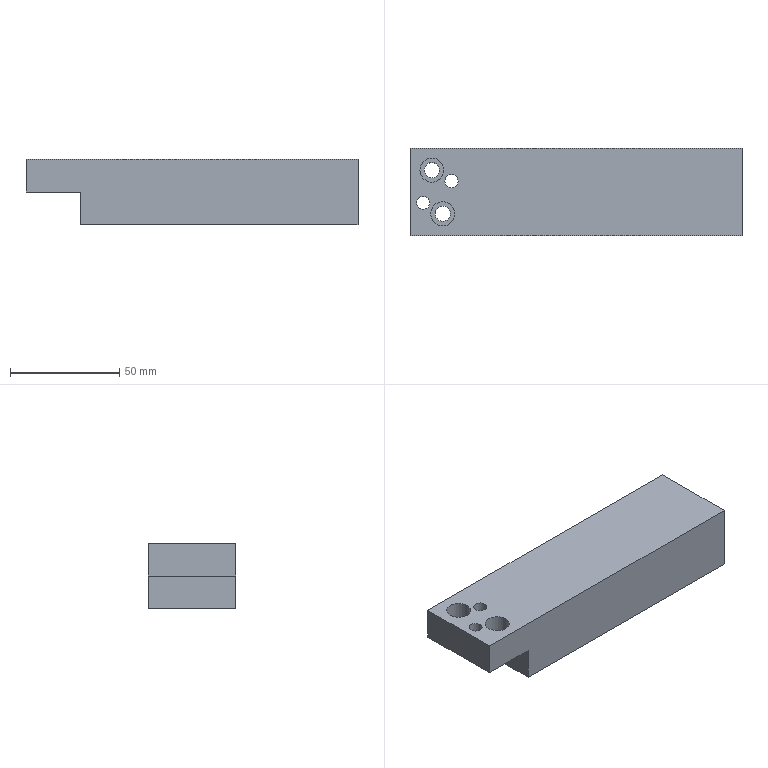Part | NX | features 22 2 | 1 solid | 16 faces | box 152 x 40 x 30 mm | volume 164266 mm3 | plane 10 | cylinder 6 | commonest cylinder face diameters 6.001 x2 7 x2 11 x2
STEP:
#1=CARTESIAN_POINT('',(905.,295.,-33.5));
#2=VERTEX_POINT('',#1);
#3=CARTESIAN_POINT('',(905.,255.,-33.5));
#4=VERTEX_POINT('',#3);
#5=CARTESIAN_POINT('',(905.,275.,-33.5));
#6=DIRECTION('',(0.,-1.,0.));
#7=VECTOR('',#6,1000.);
#8=LINE('',#5,#7);
#9=EDGE_CURVE('',#2,#4,#8,.T.);
#10=ORIENTED_EDGE('',*,*,#9,.F.);
#11=CARTESIAN_POINT('',(1032.,295.,-33.5));
#12=VERTEX_POINT('',#11);
#13=CARTESIAN_POINT('',(908.,295.,-33.5));
#14=DIRECTION('',(1.,0.,0.));
#15=VECTOR('',#14,1000.);
#16=LINE('',#13,#15);
#17=EDGE_CURVE('',#2,#12,#16,.T.);
#18=ORIENTED_EDGE('',*,*,#17,.T.);
#19=CARTESIAN_POINT('',(1032.,255.,-33.5));
#20=VERTEX_POINT('',#19);
#21=CARTESIAN_POINT('',(1032.,275.,-33.5));
#22=DIRECTION('',(0.,-1.,0.));
#23=VECTOR('',#22,1000.);
#24=LINE('',#21,#23);
#25=EDGE_CURVE('',#12,#20,#24,.T.);
#26=ORIENTED_EDGE('',*,*,#25,.T.);
#27=CARTESIAN_POINT('',(908.,255.,-33.5));
#28=DIRECTION('',(-1.,0.,0.));
#29=VECTOR('',#28,1000.);
#30=LINE('',#27,#29);
#31=EDGE_CURVE('',#20,#4,#30,.T.);
#32=ORIENTED_EDGE('',*,*,#31,.T.);
#33=EDGE_LOOP('',(#10,#18,#26,#32));
#34=FACE_BOUND('',#33,.T.);
#35=CARTESIAN_POINT('',(908.,275.,-33.5));
#36=DIRECTION('',(0.,0.,-1.));
#37=DIRECTION('',(1.,0.,0.));
#38=AXIS2_PLACEMENT_3D('',#35,#36,#37);
#39=PLANE('',#38);
#40=ADVANCED_FACE('',(#34),#39,.T.);
#41=CARTESIAN_POINT('',(889.5,265.,-3.5));
#42=VERTEX_POINT('',#41);
#43=CARTESIAN_POINT('',(895.,265.,-3.5));
#44=DIRECTION('',(0.,0.,-1.));
#45=DIRECTION('',(-1.,0.,0.));
#46=AXIS2_PLACEMENT_3D('',#43,#44,#45);
#47=CIRCLE('',#46,5.5);
#48=EDGE_CURVE('',#42,#42,#47,.T.);
#49=ORIENTED_EDGE('',*,*,#48,.T.);
#50=EDGE_LOOP('',(#49));
#51=FACE_BOUND('',#50,.T.);
#52=CARTESIAN_POINT('',(902.001,280.,-3.5));
#53=VERTEX_POINT('',#52);
#54=CARTESIAN_POINT('',(899.,280.,-3.5));
#55=DIRECTION('',(0.,0.,-1.));
#56=DIRECTION('',(1.,0.,0.));
#57=AXIS2_PLACEMENT_3D('',#54,#55,#56);
#58=CIRCLE('',#57,3.001);
#59=EDGE_CURVE('',#53,#53,#58,.T.);
#60=ORIENTED_EDGE('',*,*,#59,.T.);
#61=EDGE_LOOP('',(#60));
#62=FACE_BOUND('',#61,.T.);
#63=CARTESIAN_POINT('',(889.,270.,-3.5));
#64=VERTEX_POINT('',#63);
#65=CARTESIAN_POINT('',(886.,270.,-3.5));
#66=DIRECTION('',(0.,0.,-1.));
#67=DIRECTION('',(1.,0.,0.));
#68=AXIS2_PLACEMENT_3D('',#65,#66,#67);
#69=CIRCLE('',#68,3.001);
#70=EDGE_CURVE('',#64,#64,#69,.T.);
#71=ORIENTED_EDGE('',*,*,#70,.T.);
#72=EDGE_LOOP('',(#71));
#73=FACE_BOUND('',#72,.T.);
#74=CARTESIAN_POINT('',(880.,255.,-3.5));
#75=VERTEX_POINT('',#74);
#76=CARTESIAN_POINT('',(1032.,255.,-3.5));
#77=VERTEX_POINT('',#76);
#78=CARTESIAN_POINT('',(908.,255.,-3.5));
#79=DIRECTION('',(1.,0.,0.));
#80=VECTOR('',#79,1000.);
#81=LINE('',#78,#80);
#82=EDGE_CURVE('',#75,#77,#81,.T.);
#83=ORIENTED_EDGE('',*,*,#82,.T.);
#84=CARTESIAN_POINT('',(1032.,295.,-3.5));
#85=VERTEX_POINT('',#84);
#86=CARTESIAN_POINT('',(1032.,275.,-3.5));
#87=DIRECTION('',(0.,1.,0.));
#88=VECTOR('',#87,1000.);
#89=LINE('',#86,#88);
#90=EDGE_CURVE('',#77,#85,#89,.T.);
#91=ORIENTED_EDGE('',*,*,#90,.T.);
#92=CARTESIAN_POINT('',(880.,295.,-3.5));
#93=VERTEX_POINT('',#92);
#94=CARTESIAN_POINT('',(908.,295.,-3.5));
#95=DIRECTION('',(-1.,0.,0.));
#96=VECTOR('',#95,1000.);
#97=LINE('',#94,#96);
#98=EDGE_CURVE('',#85,#93,#97,.T.);
#99=ORIENTED_EDGE('',*,*,#98,.T.);
#100=CARTESIAN_POINT('',(880.,275.,-3.5));
#101=DIRECTION('',(0.,-1.,0.));
#102=VECTOR('',#101,1000.);
#103=LINE('',#100,#102);
#104=EDGE_CURVE('',#93,#75,#103,.T.);
#105=ORIENTED_EDGE('',*,*,#104,.T.);
#106=EDGE_LOOP('',(#83,#91,#99,#105));
#107=FACE_BOUND('',#106,.T.);
#108=CARTESIAN_POINT('',(895.5,285.,-3.5));
#109=VERTEX_POINT('',#108);
#110=CARTESIAN_POINT('',(890.,285.,-3.5));
#111=DIRECTION('',(0.,0.,1.));
#112=DIRECTION('',(1.,0.,0.));
#113=AXIS2_PLACEMENT_3D('',#110,#111,#112);
#114=CIRCLE('',#113,5.5);
#115=EDGE_CURVE('',#109,#109,#114,.T.);
#116=ORIENTED_EDGE('',*,*,#115,.F.);
#117=EDGE_LOOP('',(#116));
#118=FACE_BOUND('',#117,.T.);
#119=CARTESIAN_POINT('',(908.,275.,-3.5));
#120=DIRECTION('',(0.,0.,1.));
#121=DIRECTION('',(-1.,0.,0.));
#122=AXIS2_PLACEMENT_3D('',#119,#120,#121);
#123=PLANE('',#122);
#124=ADVANCED_FACE('',(#51,#62,#73,#107,#118),#123,.T.);
#125=CARTESIAN_POINT('',(905.,255.,-18.5));
#126=VERTEX_POINT('',#125);
#127=CARTESIAN_POINT('',(905.,295.,-18.5));
#128=VERTEX_POINT('',#127);
#129=CARTESIAN_POINT('',(905.,275.,-18.5));
#130=DIRECTION('',(0.,1.,0.));
#131=VECTOR('',#130,1000.);
#132=LINE('',#129,#131);
#133=EDGE_CURVE('',#126,#128,#132,.T.);
#134=ORIENTED_EDGE('',*,*,#133,.T.);
#135=CARTESIAN_POINT('',(905.,295.,-18.5));
#136=DIRECTION('',(0.,0.,1.));
#137=VECTOR('',#136,1000.);
#138=LINE('',#135,#137);
#139=EDGE_CURVE('',#2,#128,#138,.T.);
#140=ORIENTED_EDGE('',*,*,#139,.F.);
#141=ORIENTED_EDGE('',*,*,#9,.T.);
#142=CARTESIAN_POINT('',(905.,255.,-18.5));
#143=DIRECTION('',(0.,0.,-1.));
#144=VECTOR('',#143,1000.);
#145=LINE('',#142,#144);
#146=EDGE_CURVE('',#126,#4,#145,.T.);
#147=ORIENTED_EDGE('',*,*,#146,.F.);
#148=EDGE_LOOP('',(#134,#140,#141,#147));
#149=FACE_BOUND('',#148,.T.);
#150=CARTESIAN_POINT('',(905.,275.,-21.));
#151=DIRECTION('',(1.,0.,0.));
#152=DIRECTION('',(0.,0.,1.));
#153=AXIS2_PLACEMENT_3D('',#150,#151,#152);
#154=PLANE('',#153);
#155=ADVANCED_FACE('',(#149),#154,.F.);
#156=ORIENTED_EDGE('',*,*,#146,.T.);
#157=ORIENTED_EDGE('',*,*,#31,.F.);
#158=CARTESIAN_POINT('',(1032.,255.,-18.5));
#159=DIRECTION('',(0.,0.,1.));
#160=VECTOR('',#159,1000.);
#161=LINE('',#158,#160);
#162=EDGE_CURVE('',#20,#77,#161,.T.);
#163=ORIENTED_EDGE('',*,*,#162,.T.);
#164=ORIENTED_EDGE('',*,*,#82,.F.);
#165=CARTESIAN_POINT('',(880.,255.,-18.5));
#166=VERTEX_POINT('',#165);
#167=CARTESIAN_POINT('',(880.,255.,-18.5));
#168=DIRECTION('',(0.,0.,1.));
#169=VECTOR('',#168,1000.);
#170=LINE('',#167,#169);
#171=EDGE_CURVE('',#166,#75,#170,.T.);
#172=ORIENTED_EDGE('',*,*,#171,.F.);
#173=CARTESIAN_POINT('',(908.,255.,-18.5));
#174=DIRECTION('',(-1.,0.,0.));
#175=VECTOR('',#174,1000.);
#176=LINE('',#173,#175);
#177=EDGE_CURVE('',#126,#166,#176,.T.);
#178=ORIENTED_EDGE('',*,*,#177,.F.);
#179=EDGE_LOOP('',(#156,#157,#163,#164,#172,#178));
#180=FACE_BOUND('',#179,.T.);
#181=CARTESIAN_POINT('',(908.,255.,-18.5));
#182=DIRECTION('',(0.,-1.,0.));
#183=DIRECTION('',(0.,0.,-1.));
#184=AXIS2_PLACEMENT_3D('',#181,#182,#183);
#185=PLANE('',#184);
#186=ADVANCED_FACE('',(#180),#185,.T.);
#187=ORIENTED_EDGE('',*,*,#139,.T.);
#188=CARTESIAN_POINT('',(880.,295.,-18.5));
#189=VERTEX_POINT('',#188);
#190=CARTESIAN_POINT('',(908.,295.,-18.5));
#191=DIRECTION('',(1.,0.,0.));
#192=VECTOR('',#191,1000.);
#193=LINE('',#190,#192);
#194=EDGE_CURVE('',#189,#128,#193,.T.);
#195=ORIENTED_EDGE('',*,*,#194,.F.);
#196=CARTESIAN_POINT('',(880.,295.,-18.5));
#197=DIRECTION('',(0.,0.,1.));
#198=VECTOR('',#197,1000.);
#199=LINE('',#196,#198);
#200=EDGE_CURVE('',#189,#93,#199,.T.);
#201=ORIENTED_EDGE('',*,*,#200,.T.);
#202=ORIENTED_EDGE('',*,*,#98,.F.);
#203=CARTESIAN_POINT('',(1032.,295.,-18.5));
#204=DIRECTION('',(0.,0.,1.));
#205=VECTOR('',#204,1000.);
#206=LINE('',#203,#205);
#207=EDGE_CURVE('',#12,#85,#206,.T.);
#208=ORIENTED_EDGE('',*,*,#207,.F.);
#209=ORIENTED_EDGE('',*,*,#17,.F.);
#210=EDGE_LOOP('',(#187,#195,#201,#202,#208,#209));
#211=FACE_BOUND('',#210,.T.);
#212=CARTESIAN_POINT('',(908.,295.,-18.5));
#213=DIRECTION('',(0.,1.,0.));
#214=DIRECTION('',(0.,0.,1.));
#215=AXIS2_PLACEMENT_3D('',#212,#213,#214);
#216=PLANE('',#215);
#217=ADVANCED_FACE('',(#211),#216,.T.);
#218=ORIENTED_EDGE('',*,*,#90,.F.);
#219=ORIENTED_EDGE('',*,*,#162,.F.);
#220=ORIENTED_EDGE('',*,*,#25,.F.);
#221=ORIENTED_EDGE('',*,*,#207,.T.);
#222=EDGE_LOOP('',(#218,#219,#220,#221));
#223=FACE_BOUND('',#222,.T.);
#224=CARTESIAN_POINT('',(1032.,275.,-18.5));
#225=DIRECTION('',(1.,0.,0.));
#226=DIRECTION('',(0.,0.,1.));
#227=AXIS2_PLACEMENT_3D('',#224,#225,#226);
#228=PLANE('',#227);
#229=ADVANCED_FACE('',(#223),#228,.T.);
#230=ORIENTED_EDGE('',*,*,#200,.F.);
#231=CARTESIAN_POINT('',(880.,275.,-18.5));
#232=DIRECTION('',(0.,1.,0.));
#233=VECTOR('',#232,1000.);
#234=LINE('',#231,#233);
#235=EDGE_CURVE('',#166,#189,#234,.T.);
#236=ORIENTED_EDGE('',*,*,#235,.F.);
#237=ORIENTED_EDGE('',*,*,#171,.T.);
#238=ORIENTED_EDGE('',*,*,#104,.F.);
#239=EDGE_LOOP('',(#230,#236,#237,#238));
#240=FACE_BOUND('',#239,.T.);
#241=CARTESIAN_POINT('',(880.,275.,-18.5));
#242=DIRECTION('',(-1.,0.,0.));
#243=DIRECTION('',(0.,0.,-1.));
#244=AXIS2_PLACEMENT_3D('',#241,#242,#243);
#245=PLANE('',#244);
#246=ADVANCED_FACE('',(#240),#245,.T.);
#247=CARTESIAN_POINT('',(891.5,265.,-18.5));
#248=VERTEX_POINT('',#247);
#249=CARTESIAN_POINT('',(895.,265.,-18.5));
#250=DIRECTION('',(0.,0.,1.));
#251=DIRECTION('',(-1.,0.,0.));
#252=AXIS2_PLACEMENT_3D('',#249,#250,#251);
#253=CIRCLE('',#252,3.5);
#254=EDGE_CURVE('',#248,#248,#253,.T.);
#255=ORIENTED_EDGE('',*,*,#254,.T.);
#256=EDGE_LOOP('',(#255));
#257=FACE_BOUND('',#256,.T.);
#258=CARTESIAN_POINT('',(896.,280.,-18.5));
#259=VERTEX_POINT('',#258);
#260=CARTESIAN_POINT('',(899.,280.,-18.5));
#261=DIRECTION('',(0.,0.,1.));
#262=DIRECTION('',(-1.,0.,0.));
#263=AXIS2_PLACEMENT_3D('',#260,#261,#262);
#264=CIRCLE('',#263,3.001);
#265=EDGE_CURVE('',#259,#259,#264,.T.);
#266=ORIENTED_EDGE('',*,*,#265,.T.);
#267=EDGE_LOOP('',(#266));
#268=FACE_BOUND('',#267,.T.);
#269=CARTESIAN_POINT('',(882.999,270.,-18.5));
#270=VERTEX_POINT('',#269);
#271=CARTESIAN_POINT('',(886.,270.,-18.5));
#272=DIRECTION('',(0.,0.,1.));
#273=DIRECTION('',(-1.,0.,0.));
#274=AXIS2_PLACEMENT_3D('',#271,#272,#273);
#275=CIRCLE('',#274,3.001);
#276=EDGE_CURVE('',#270,#270,#275,.T.);
#277=ORIENTED_EDGE('',*,*,#276,.T.);
#278=EDGE_LOOP('',(#277));
#279=FACE_BOUND('',#278,.T.);
#280=CARTESIAN_POINT('',(886.5,285.,-18.5));
#281=VERTEX_POINT('',#280);
#282=CARTESIAN_POINT('',(890.,285.,-18.5));
#283=DIRECTION('',(0.,0.,1.));
#284=DIRECTION('',(-1.,0.,0.));
#285=AXIS2_PLACEMENT_3D('',#282,#283,#284);
#286=CIRCLE('',#285,3.5);
#287=EDGE_CURVE('',#281,#281,#286,.T.);
#288=ORIENTED_EDGE('',*,*,#287,.T.);
#289=EDGE_LOOP('',(#288));
#290=FACE_BOUND('',#289,.T.);
#291=ORIENTED_EDGE('',*,*,#177,.T.);
#292=ORIENTED_EDGE('',*,*,#235,.T.);
#293=ORIENTED_EDGE('',*,*,#194,.T.);
#294=ORIENTED_EDGE('',*,*,#133,.F.);
#295=EDGE_LOOP('',(#291,#292,#293,#294));
#296=FACE_BOUND('',#295,.T.);
#297=CARTESIAN_POINT('',(908.,275.,-18.5));
#298=DIRECTION('',(0.,0.,-1.));
#299=DIRECTION('',(1.,0.,0.));
#300=AXIS2_PLACEMENT_3D('',#297,#298,#299);
#301=PLANE('',#300);
#302=ADVANCED_FACE('',(#257,#268,#279,#290,#296),#301,.T.);
#303=ORIENTED_EDGE('',*,*,#287,.F.);
#304=EDGE_LOOP('',(#303));
#305=FACE_BOUND('',#304,.T.);
#306=CARTESIAN_POINT('',(886.5,285.,-13.5));
#307=VERTEX_POINT('',#306);
#308=CARTESIAN_POINT('',(890.,285.,-13.5));
#309=DIRECTION('',(0.,0.,1.));
#310=DIRECTION('',(-1.,0.,0.));
#311=AXIS2_PLACEMENT_3D('',#308,#309,#310);
#312=CIRCLE('',#311,3.5);
#313=EDGE_CURVE('',#307,#307,#312,.T.);
#314=ORIENTED_EDGE('',*,*,#313,.T.);
#315=EDGE_LOOP('',(#314));
#316=FACE_BOUND('',#315,.T.);
#317=CARTESIAN_POINT('',(890.,285.,-1.5));
#318=DIRECTION('',(0.,0.,-1.));
#319=DIRECTION('',(-1.,0.,0.));
#320=AXIS2_PLACEMENT_3D('',#317,#318,#319);
#321=CYLINDRICAL_SURFACE('',#320,3.5);
#322=ADVANCED_FACE('',(#305,#316),#321,.F.);
#323=ORIENTED_EDGE('',*,*,#313,.F.);
#324=EDGE_LOOP('',(#323));
#325=FACE_BOUND('',#324,.T.);
#326=CARTESIAN_POINT('',(895.5,285.,-13.5));
#327=VERTEX_POINT('',#326);
#328=CARTESIAN_POINT('',(890.,285.,-13.5));
#329=DIRECTION('',(0.,0.,1.));
#330=DIRECTION('',(1.,0.,0.));
#331=AXIS2_PLACEMENT_3D('',#328,#329,#330);
#332=CIRCLE('',#331,5.5);
#333=EDGE_CURVE('',#327,#327,#332,.T.);
#334=ORIENTED_EDGE('',*,*,#333,.T.);
#335=EDGE_LOOP('',(#334));
#336=FACE_BOUND('',#335,.T.);
#337=CARTESIAN_POINT('',(890.,285.,-13.5));
#338=DIRECTION('',(0.,0.,-1.));
#339=DIRECTION('',(1.,0.,0.));
#340=AXIS2_PLACEMENT_3D('',#337,#338,#339);
#341=PLANE('',#340);
#342=ADVANCED_FACE('',(#325,#336),#341,.F.);
#343=ORIENTED_EDGE('',*,*,#333,.F.);
#344=EDGE_LOOP('',(#343));
#345=FACE_BOUND('',#344,.T.);
#346=ORIENTED_EDGE('',*,*,#115,.T.);
#347=EDGE_LOOP('',(#346));
#348=FACE_BOUND('',#347,.T.);
#349=CARTESIAN_POINT('',(890.,285.,-3.5));
#350=DIRECTION('',(0.,0.,-1.));
#351=DIRECTION('',(-1.,0.,0.));
#352=AXIS2_PLACEMENT_3D('',#349,#350,#351);
#353=CYLINDRICAL_SURFACE('',#352,5.5);
#354=ADVANCED_FACE('',(#345,#348),#353,.F.);
#355=ORIENTED_EDGE('',*,*,#70,.F.);
#356=EDGE_LOOP('',(#355));
#357=FACE_BOUND('',#356,.T.);
#358=ORIENTED_EDGE('',*,*,#276,.F.);
#359=EDGE_LOOP('',(#358));
#360=FACE_BOUND('',#359,.T.);
#361=CARTESIAN_POINT('',(886.,270.,-1.5));
#362=DIRECTION('',(0.,0.,-1.));
#363=DIRECTION('',(-1.,0.,0.));
#364=AXIS2_PLACEMENT_3D('',#361,#362,#363);
#365=CYLINDRICAL_SURFACE('',#364,3.001);
#366=ADVANCED_FACE('',(#357,#360),#365,.F.);
#367=ORIENTED_EDGE('',*,*,#59,.F.);
#368=EDGE_LOOP('',(#367));
#369=FACE_BOUND('',#368,.T.);
#370=ORIENTED_EDGE('',*,*,#265,.F.);
#371=EDGE_LOOP('',(#370));
#372=FACE_BOUND('',#371,.T.);
#373=CARTESIAN_POINT('',(899.,280.,-1.5));
#374=DIRECTION('',(0.,0.,-1.));
#375=DIRECTION('',(1.,0.,0.));
#376=AXIS2_PLACEMENT_3D('',#373,#374,#375);
#377=CYLINDRICAL_SURFACE('',#376,3.001);
#378=ADVANCED_FACE('',(#369,#372),#377,.F.);
#379=ORIENTED_EDGE('',*,*,#254,.F.);
#380=EDGE_LOOP('',(#379));
#381=FACE_BOUND('',#380,.T.);
#382=CARTESIAN_POINT('',(898.5,265.,-13.5));
#383=VERTEX_POINT('',#382);
#384=CARTESIAN_POINT('',(895.,265.,-13.5));
#385=DIRECTION('',(0.,0.,-1.));
#386=DIRECTION('',(1.,0.,0.));
#387=AXIS2_PLACEMENT_3D('',#384,#385,#386);
#388=CIRCLE('',#387,3.5);
#389=EDGE_CURVE('',#383,#383,#388,.T.);
#390=ORIENTED_EDGE('',*,*,#389,.F.);
#391=EDGE_LOOP('',(#390));
#392=FACE_BOUND('',#391,.T.);
#393=CARTESIAN_POINT('',(895.,265.,-1.5));
#394=DIRECTION('',(0.,0.,-1.));
#395=DIRECTION('',(1.,0.,0.));
#396=AXIS2_PLACEMENT_3D('',#393,#394,#395);
#397=CYLINDRICAL_SURFACE('',#396,3.5);
#398=ADVANCED_FACE('',(#381,#392),#397,.F.);
#399=ORIENTED_EDGE('',*,*,#389,.T.);
#400=EDGE_LOOP('',(#399));
#401=FACE_BOUND('',#400,.T.);
#402=CARTESIAN_POINT('',(889.5,265.,-13.5));
#403=VERTEX_POINT('',#402);
#404=CARTESIAN_POINT('',(895.,265.,-13.5));
#405=DIRECTION('',(0.,0.,-1.));
#406=DIRECTION('',(-1.,0.,0.));
#407=AXIS2_PLACEMENT_3D('',#404,#405,#406);
#408=CIRCLE('',#407,5.5);
#409=EDGE_CURVE('',#403,#403,#408,.T.);
#410=ORIENTED_EDGE('',*,*,#409,.F.);
#411=EDGE_LOOP('',(#410));
#412=FACE_BOUND('',#411,.T.);
#413=CARTESIAN_POINT('',(895.,265.,-13.5));
#414=DIRECTION('',(0.,0.,-1.));
#415=DIRECTION('',(-1.,0.,0.));
#416=AXIS2_PLACEMENT_3D('',#413,#414,#415);
#417=PLANE('',#416);
#418=ADVANCED_FACE('',(#401,#412),#417,.F.);
#419=ORIENTED_EDGE('',*,*,#409,.T.);
#420=EDGE_LOOP('',(#419));
#421=FACE_BOUND('',#420,.T.);
#422=ORIENTED_EDGE('',*,*,#48,.F.);
#423=EDGE_LOOP('',(#422));
#424=FACE_BOUND('',#423,.T.);
#425=CARTESIAN_POINT('',(895.,265.,-3.5));
#426=DIRECTION('',(0.,0.,-1.));
#427=DIRECTION('',(1.,0.,0.));
#428=AXIS2_PLACEMENT_3D('',#425,#426,#427);
#429=CYLINDRICAL_SURFACE('',#428,5.5);
#430=ADVANCED_FACE('',(#421,#424),#429,.F.);
#431=CLOSED_SHELL('',(#40,#124,#155,#186,#217,#229,#246,#302,#322,#342,#354,#366,#378,#398,#418,#430));
#432=MANIFOLD_SOLID_BREP('',#431);
#433=(LENGTH_UNIT()NAMED_UNIT(*)SI_UNIT(.MILLI.,.METRE.));
#434=UNCERTAINTY_MEASURE_WITH_UNIT(LENGTH_MEASURE(0.00001),#433,'','');
#435=(NAMED_UNIT(*)PLANE_ANGLE_UNIT()SI_UNIT($,.RADIAN.));
#436=(NAMED_UNIT(*)SI_UNIT($,.STERADIAN.)SOLID_ANGLE_UNIT());
#437=(GEOMETRIC_REPRESENTATION_CONTEXT(3)GLOBAL_UNCERTAINTY_ASSIGNED_CONTEXT((#434))GLOBAL_UNIT_ASSIGNED_CONTEXT((#433,#435,#436))REPRESENTATION_CONTEXT('',''));
#438=ADVANCED_BREP_SHAPE_REPRESENTATION('',(#432),#437);